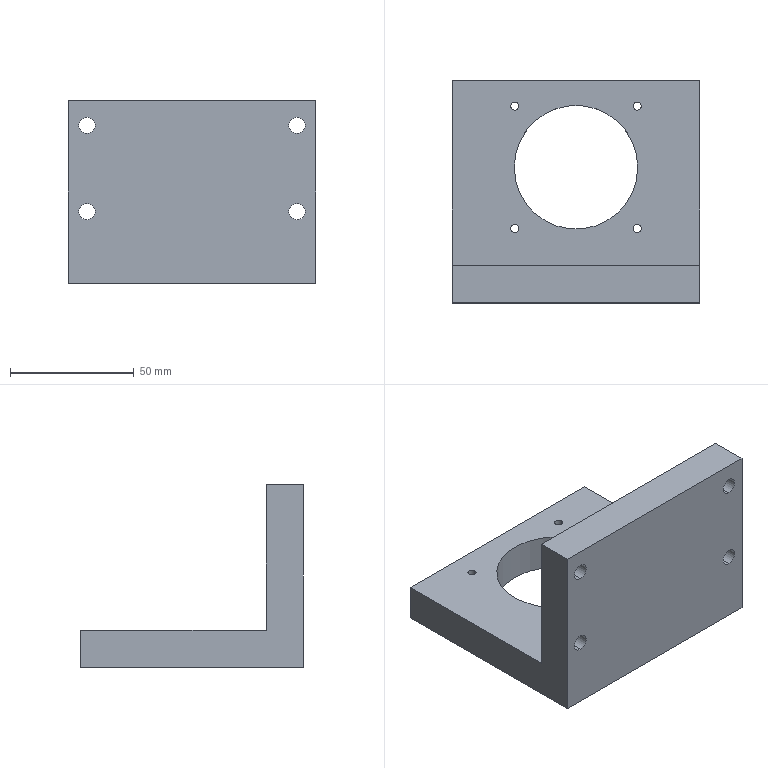Part | SolidWorks | features BaseBody 1 | 1 solid | 46 faces | box 100 x 90 x 74 mm | volume 189827 mm3 | cylinder 26 | plane 12 | cone 8 | commonest cylinder face diameters 3.3 x8 6.6 x8 11 x8 50 x2
STEP:
#1=CARTESIAN_POINT('',(26.399,34.749,0.));
#2=VERTEX_POINT('',#1);
#3=CARTESIAN_POINT('',(23.099,34.749,0.));
#4=VERTEX_POINT('',#3);
#5=CARTESIAN_POINT('',(24.749,34.749,0.));
#6=DIRECTION('',(0.,0.,-1.));
#7=DIRECTION('',(1.,0.,0.));
#8=AXIS2_PLACEMENT_3D('',#5,#6,#7);
#9=CIRCLE('',#8,1.65);
#10=EDGE_CURVE('',#2,#4,#9,.T.);
#11=ORIENTED_EDGE('',*,*,#10,.T.);
#12=CARTESIAN_POINT('',(23.099,34.749,15.));
#13=VERTEX_POINT('',#12);
#14=CARTESIAN_POINT('',(23.099,34.749,0.));
#15=DIRECTION('',(0.,0.,1.));
#16=VECTOR('',#15,1000.);
#17=LINE('',#14,#16);
#18=EDGE_CURVE('',#4,#13,#17,.T.);
#19=ORIENTED_EDGE('',*,*,#18,.T.);
#20=CARTESIAN_POINT('',(26.399,34.749,15.));
#21=VERTEX_POINT('',#20);
#22=CARTESIAN_POINT('',(24.749,34.749,15.));
#23=DIRECTION('',(0.,0.,1.));
#24=DIRECTION('',(1.,0.,0.));
#25=AXIS2_PLACEMENT_3D('',#22,#23,#24);
#26=CIRCLE('',#25,1.65);
#27=EDGE_CURVE('',#13,#21,#26,.T.);
#28=ORIENTED_EDGE('',*,*,#27,.T.);
#29=CARTESIAN_POINT('',(26.399,34.749,0.));
#30=DIRECTION('',(0.,0.,1.));
#31=VECTOR('',#30,1000.);
#32=LINE('',#29,#31);
#33=EDGE_CURVE('',#2,#21,#32,.T.);
#34=ORIENTED_EDGE('',*,*,#33,.F.);
#35=EDGE_LOOP('',(#11,#19,#28,#34));
#36=FACE_OUTER_BOUND('',#35,.T.);
#37=CARTESIAN_POINT('',(24.749,34.749,0.));
#38=DIRECTION('',(0.,0.,1.));
#39=DIRECTION('',(1.,0.,0.));
#40=AXIS2_PLACEMENT_3D('',#37,#38,#39);
#41=CYLINDRICAL_SURFACE('',#40,1.65);
#42=ADVANCED_FACE('',(#36),#41,.F.);
#43=CARTESIAN_POINT('',(25.,10.,0.));
#44=VERTEX_POINT('',#43);
#45=CARTESIAN_POINT('',(-25.,10.,0.));
#46=VERTEX_POINT('',#45);
#47=CARTESIAN_POINT('',(0.,10.,0.));
#48=DIRECTION('',(0.,0.,-1.));
#49=DIRECTION('',(1.,0.,0.));
#50=AXIS2_PLACEMENT_3D('',#47,#48,#49);
#51=CIRCLE('',#50,25.);
#52=EDGE_CURVE('',#44,#46,#51,.T.);
#53=ORIENTED_EDGE('',*,*,#52,.T.);
#54=CARTESIAN_POINT('',(-25.,10.,15.));
#55=VERTEX_POINT('',#54);
#56=CARTESIAN_POINT('',(-25.,10.,0.));
#57=DIRECTION('',(0.,0.,1.));
#58=VECTOR('',#57,1000.);
#59=LINE('',#56,#58);
#60=EDGE_CURVE('',#46,#55,#59,.T.);
#61=ORIENTED_EDGE('',*,*,#60,.T.);
#62=CARTESIAN_POINT('',(25.,10.,15.));
#63=VERTEX_POINT('',#62);
#64=CARTESIAN_POINT('',(0.,10.,15.));
#65=DIRECTION('',(0.,0.,-1.));
#66=DIRECTION('',(1.,0.,0.));
#67=AXIS2_PLACEMENT_3D('',#64,#65,#66);
#68=CIRCLE('',#67,25.);
#69=EDGE_CURVE('',#63,#55,#68,.T.);
#70=ORIENTED_EDGE('',*,*,#69,.F.);
#71=CARTESIAN_POINT('',(25.,10.,0.));
#72=DIRECTION('',(0.,0.,1.));
#73=VECTOR('',#72,1000.);
#74=LINE('',#71,#73);
#75=EDGE_CURVE('',#44,#63,#74,.T.);
#76=ORIENTED_EDGE('',*,*,#75,.F.);
#77=EDGE_LOOP('',(#53,#61,#70,#76));
#78=FACE_OUTER_BOUND('',#77,.T.);
#79=CARTESIAN_POINT('',(0.,10.,0.));
#80=DIRECTION('',(0.,0.,1.));
#81=DIRECTION('',(1.,0.,0.));
#82=AXIS2_PLACEMENT_3D('',#79,#80,#81);
#83=CYLINDRICAL_SURFACE('',#82,25.);
#84=ADVANCED_FACE('',(#78),#83,.F.);
#85=CARTESIAN_POINT('',(26.399,-14.749,0.));
#86=VERTEX_POINT('',#85);
#87=CARTESIAN_POINT('',(23.099,-14.749,0.));
#88=VERTEX_POINT('',#87);
#89=CARTESIAN_POINT('',(24.749,-14.749,0.));
#90=DIRECTION('',(0.,0.,-1.));
#91=DIRECTION('',(1.,0.,0.));
#92=AXIS2_PLACEMENT_3D('',#89,#90,#91);
#93=CIRCLE('',#92,1.65);
#94=EDGE_CURVE('',#86,#88,#93,.T.);
#95=ORIENTED_EDGE('',*,*,#94,.T.);
#96=CARTESIAN_POINT('',(23.099,-14.749,15.));
#97=VERTEX_POINT('',#96);
#98=CARTESIAN_POINT('',(23.099,-14.749,0.));
#99=DIRECTION('',(0.,0.,1.));
#100=VECTOR('',#99,1000.);
#101=LINE('',#98,#100);
#102=EDGE_CURVE('',#88,#97,#101,.T.);
#103=ORIENTED_EDGE('',*,*,#102,.T.);
#104=CARTESIAN_POINT('',(26.399,-14.749,15.));
#105=VERTEX_POINT('',#104);
#106=CARTESIAN_POINT('',(24.749,-14.749,15.));
#107=DIRECTION('',(0.,0.,-1.));
#108=DIRECTION('',(1.,0.,0.));
#109=AXIS2_PLACEMENT_3D('',#106,#107,#108);
#110=CIRCLE('',#109,1.65);
#111=EDGE_CURVE('',#105,#97,#110,.T.);
#112=ORIENTED_EDGE('',*,*,#111,.F.);
#113=CARTESIAN_POINT('',(26.399,-14.749,0.));
#114=DIRECTION('',(0.,0.,1.));
#115=VECTOR('',#114,1000.);
#116=LINE('',#113,#115);
#117=EDGE_CURVE('',#86,#105,#116,.T.);
#118=ORIENTED_EDGE('',*,*,#117,.F.);
#119=EDGE_LOOP('',(#95,#103,#112,#118));
#120=FACE_OUTER_BOUND('',#119,.T.);
#121=CARTESIAN_POINT('',(24.749,-14.749,0.));
#122=DIRECTION('',(0.,0.,1.));
#123=DIRECTION('',(1.,0.,0.));
#124=AXIS2_PLACEMENT_3D('',#121,#122,#123);
#125=CYLINDRICAL_SURFACE('',#124,1.65);
#126=ADVANCED_FACE('',(#120),#125,.F.);
#127=CARTESIAN_POINT('',(-23.099,-14.749,0.));
#128=VERTEX_POINT('',#127);
#129=CARTESIAN_POINT('',(-26.399,-14.749,0.));
#130=VERTEX_POINT('',#129);
#131=CARTESIAN_POINT('',(-24.749,-14.749,0.));
#132=DIRECTION('',(0.,0.,-1.));
#133=DIRECTION('',(1.,0.,0.));
#134=AXIS2_PLACEMENT_3D('',#131,#132,#133);
#135=CIRCLE('',#134,1.65);
#136=EDGE_CURVE('',#128,#130,#135,.T.);
#137=ORIENTED_EDGE('',*,*,#136,.T.);
#138=CARTESIAN_POINT('',(-26.399,-14.749,15.));
#139=VERTEX_POINT('',#138);
#140=CARTESIAN_POINT('',(-26.399,-14.749,0.));
#141=DIRECTION('',(0.,0.,1.));
#142=VECTOR('',#141,1000.);
#143=LINE('',#140,#142);
#144=EDGE_CURVE('',#130,#139,#143,.T.);
#145=ORIENTED_EDGE('',*,*,#144,.T.);
#146=CARTESIAN_POINT('',(-23.099,-14.749,15.));
#147=VERTEX_POINT('',#146);
#148=CARTESIAN_POINT('',(-24.749,-14.749,15.));
#149=DIRECTION('',(0.,0.,-1.));
#150=DIRECTION('',(1.,0.,0.));
#151=AXIS2_PLACEMENT_3D('',#148,#149,#150);
#152=CIRCLE('',#151,1.65);
#153=EDGE_CURVE('',#147,#139,#152,.T.);
#154=ORIENTED_EDGE('',*,*,#153,.F.);
#155=CARTESIAN_POINT('',(-23.099,-14.749,0.));
#156=DIRECTION('',(0.,0.,1.));
#157=VECTOR('',#156,1000.);
#158=LINE('',#155,#157);
#159=EDGE_CURVE('',#128,#147,#158,.T.);
#160=ORIENTED_EDGE('',*,*,#159,.F.);
#161=EDGE_LOOP('',(#137,#145,#154,#160));
#162=FACE_OUTER_BOUND('',#161,.T.);
#163=CARTESIAN_POINT('',(-24.749,-14.749,0.));
#164=DIRECTION('',(0.,0.,1.));
#165=DIRECTION('',(1.,0.,0.));
#166=AXIS2_PLACEMENT_3D('',#163,#164,#165);
#167=CYLINDRICAL_SURFACE('',#166,1.65);
#168=ADVANCED_FACE('',(#162),#167,.F.);
#169=CARTESIAN_POINT('',(-23.099,34.749,0.));
#170=VERTEX_POINT('',#169);
#171=CARTESIAN_POINT('',(-26.399,34.749,0.));
#172=VERTEX_POINT('',#171);
#173=CARTESIAN_POINT('',(-24.749,34.749,0.));
#174=DIRECTION('',(0.,0.,-1.));
#175=DIRECTION('',(1.,0.,0.));
#176=AXIS2_PLACEMENT_3D('',#173,#174,#175);
#177=CIRCLE('',#176,1.65);
#178=EDGE_CURVE('',#170,#172,#177,.T.);
#179=ORIENTED_EDGE('',*,*,#178,.T.);
#180=CARTESIAN_POINT('',(-26.399,34.749,15.));
#181=VERTEX_POINT('',#180);
#182=CARTESIAN_POINT('',(-26.399,34.749,0.));
#183=DIRECTION('',(0.,0.,1.));
#184=VECTOR('',#183,1000.);
#185=LINE('',#182,#184);
#186=EDGE_CURVE('',#172,#181,#185,.T.);
#187=ORIENTED_EDGE('',*,*,#186,.T.);
#188=CARTESIAN_POINT('',(-23.099,34.749,15.));
#189=VERTEX_POINT('',#188);
#190=CARTESIAN_POINT('',(-24.749,34.749,15.));
#191=DIRECTION('',(0.,0.,-1.));
#192=DIRECTION('',(1.,0.,0.));
#193=AXIS2_PLACEMENT_3D('',#190,#191,#192);
#194=CIRCLE('',#193,1.65);
#195=EDGE_CURVE('',#189,#181,#194,.T.);
#196=ORIENTED_EDGE('',*,*,#195,.F.);
#197=CARTESIAN_POINT('',(-23.099,34.749,0.));
#198=DIRECTION('',(0.,0.,1.));
#199=VECTOR('',#198,1000.);
#200=LINE('',#197,#199);
#201=EDGE_CURVE('',#170,#189,#200,.T.);
#202=ORIENTED_EDGE('',*,*,#201,.F.);
#203=EDGE_LOOP('',(#179,#187,#196,#202));
#204=FACE_OUTER_BOUND('',#203,.T.);
#205=CARTESIAN_POINT('',(-24.749,34.749,0.));
#206=DIRECTION('',(0.,0.,1.));
#207=DIRECTION('',(1.,0.,0.));
#208=AXIS2_PLACEMENT_3D('',#205,#206,#207);
#209=CYLINDRICAL_SURFACE('',#208,1.65);
#210=ADVANCED_FACE('',(#204),#209,.F.);
#211=CARTESIAN_POINT('',(42.5,-30.025,23.5));
#212=VERTEX_POINT('',#211);
#213=CARTESIAN_POINT('',(48.,-30.025,29.));
#214=VERTEX_POINT('',#213);
#215=CARTESIAN_POINT('',(42.5,-30.025,29.));
#216=DIRECTION('',(0.,-1.,0.));
#217=DIRECTION('',(0.,0.,1.));
#218=AXIS2_PLACEMENT_3D('',#215,#216,#217);
#219=CIRCLE('',#218,5.5);
#220=EDGE_CURVE('',#212,#214,#219,.T.);
#221=ORIENTED_EDGE('',*,*,#220,.T.);
#222=CARTESIAN_POINT('',(48.025,-30.,29.));
#223=VERTEX_POINT('',#222);
#224=CARTESIAN_POINT('',(48.,-30.025,29.));
#225=DIRECTION('',(0.7071,0.7071,0.));
#226=VECTOR('',#225,1000.);
#227=LINE('',#224,#226);
#228=EDGE_CURVE('',#214,#223,#227,.T.);
#229=ORIENTED_EDGE('',*,*,#228,.T.);
#230=CARTESIAN_POINT('',(36.975,-30.,29.));
#231=VERTEX_POINT('',#230);
#232=CARTESIAN_POINT('',(42.5,-30.,29.));
#233=DIRECTION('',(0.,1.,0.));
#234=DIRECTION('',(-1.,0.,0.));
#235=AXIS2_PLACEMENT_3D('',#232,#233,#234);
#236=CIRCLE('',#235,5.525);
#237=EDGE_CURVE('',#223,#231,#236,.T.);
#238=ORIENTED_EDGE('',*,*,#237,.T.);
#239=CARTESIAN_POINT('',(37.,-30.025,29.));
#240=VERTEX_POINT('',#239);
#241=CARTESIAN_POINT('',(37.,-30.025,29.));
#242=DIRECTION('',(-0.7071,0.7071,0.));
#243=VECTOR('',#242,1000.);
#244=LINE('',#241,#243);
#245=EDGE_CURVE('',#240,#231,#244,.T.);
#246=ORIENTED_EDGE('',*,*,#245,.F.);
#247=CARTESIAN_POINT('',(42.5,-30.025,29.));
#248=DIRECTION('',(0.,-1.,0.));
#249=DIRECTION('',(0.,0.,1.));
#250=AXIS2_PLACEMENT_3D('',#247,#248,#249);
#251=CIRCLE('',#250,5.5);
#252=EDGE_CURVE('',#240,#212,#251,.T.);
#253=ORIENTED_EDGE('',*,*,#252,.T.);
#254=EDGE_LOOP('',(#221,#229,#238,#246,#253));
#255=FACE_OUTER_BOUND('',#254,.T.);
#256=CARTESIAN_POINT('',(42.5,-30.025,29.));
#257=DIRECTION('',(0.,1.,0.));
#258=DIRECTION('',(-1.,0.,0.));
#259=AXIS2_PLACEMENT_3D('',#256,#257,#258);
#260=CONICAL_SURFACE('',#259,5.5,0.7854);
#261=ADVANCED_FACE('',(#255),#260,.F.);
#262=CARTESIAN_POINT('',(42.5,-30.025,58.5));
#263=VERTEX_POINT('',#262);
#264=CARTESIAN_POINT('',(48.,-30.025,64.));
#265=VERTEX_POINT('',#264);
#266=CARTESIAN_POINT('',(42.5,-30.025,64.));
#267=DIRECTION('',(0.,-1.,0.));
#268=DIRECTION('',(0.,0.,1.));
#269=AXIS2_PLACEMENT_3D('',#266,#267,#268);
#270=CIRCLE('',#269,5.5);
#271=EDGE_CURVE('',#263,#265,#270,.T.);
#272=ORIENTED_EDGE('',*,*,#271,.T.);
#273=CARTESIAN_POINT('',(48.025,-30.,64.));
#274=VERTEX_POINT('',#273);
#275=CARTESIAN_POINT('',(48.,-30.025,64.));
#276=DIRECTION('',(0.7071,0.7071,0.));
#277=VECTOR('',#276,1000.);
#278=LINE('',#275,#277);
#279=EDGE_CURVE('',#265,#274,#278,.T.);
#280=ORIENTED_EDGE('',*,*,#279,.T.);
#281=CARTESIAN_POINT('',(36.975,-30.,64.));
#282=VERTEX_POINT('',#281);
#283=CARTESIAN_POINT('',(42.5,-30.,64.));
#284=DIRECTION('',(0.,1.,0.));
#285=DIRECTION('',(-1.,0.,0.));
#286=AXIS2_PLACEMENT_3D('',#283,#284,#285);
#287=CIRCLE('',#286,5.525);
#288=EDGE_CURVE('',#274,#282,#287,.T.);
#289=ORIENTED_EDGE('',*,*,#288,.T.);
#290=CARTESIAN_POINT('',(37.,-30.025,64.));
#291=VERTEX_POINT('',#290);
#292=CARTESIAN_POINT('',(37.,-30.025,64.));
#293=DIRECTION('',(-0.7071,0.7071,0.));
#294=VECTOR('',#293,1000.);
#295=LINE('',#292,#294);
#296=EDGE_CURVE('',#291,#282,#295,.T.);
#297=ORIENTED_EDGE('',*,*,#296,.F.);
#298=CARTESIAN_POINT('',(42.5,-30.025,64.));
#299=DIRECTION('',(0.,-1.,0.));
#300=DIRECTION('',(0.,0.,1.));
#301=AXIS2_PLACEMENT_3D('',#298,#299,#300);
#302=CIRCLE('',#301,5.5);
#303=EDGE_CURVE('',#291,#263,#302,.T.);
#304=ORIENTED_EDGE('',*,*,#303,.T.);
#305=EDGE_LOOP('',(#272,#280,#289,#297,#304));
#306=FACE_OUTER_BOUND('',#305,.T.);
#307=CARTESIAN_POINT('',(42.5,-30.025,64.));
#308=DIRECTION('',(0.,1.,0.));
#309=DIRECTION('',(-1.,0.,0.));
#310=AXIS2_PLACEMENT_3D('',#307,#308,#309);
#311=CONICAL_SURFACE('',#310,5.5,0.7854);
#312=ADVANCED_FACE('',(#306),#311,.F.);
#313=CARTESIAN_POINT('',(-42.5,-30.025,58.5));
#314=VERTEX_POINT('',#313);
#315=CARTESIAN_POINT('',(-37.,-30.025,64.));
#316=VERTEX_POINT('',#315);
#317=CARTESIAN_POINT('',(-42.5,-30.025,64.));
#318=DIRECTION('',(0.,-1.,0.));
#319=DIRECTION('',(0.,0.,1.));
#320=AXIS2_PLACEMENT_3D('',#317,#318,#319);
#321=CIRCLE('',#320,5.5);
#322=EDGE_CURVE('',#314,#316,#321,.T.);
#323=ORIENTED_EDGE('',*,*,#322,.T.);
#324=CARTESIAN_POINT('',(-36.975,-30.,64.));
#325=VERTEX_POINT('',#324);
#326=CARTESIAN_POINT('',(-37.,-30.025,64.));
#327=DIRECTION('',(0.7071,0.7071,0.));
#328=VECTOR('',#327,1000.);
#329=LINE('',#326,#328);
#330=EDGE_CURVE('',#316,#325,#329,.T.);
#331=ORIENTED_EDGE('',*,*,#330,.T.);
#332=CARTESIAN_POINT('',(-48.025,-30.,64.));
#333=VERTEX_POINT('',#332);
#334=CARTESIAN_POINT('',(-42.5,-30.,64.));
#335=DIRECTION('',(0.,1.,0.));
#336=DIRECTION('',(-1.,0.,0.));
#337=AXIS2_PLACEMENT_3D('',#334,#335,#336);
#338=CIRCLE('',#337,5.525);
#339=EDGE_CURVE('',#325,#333,#338,.T.);
#340=ORIENTED_EDGE('',*,*,#339,.T.);
#341=CARTESIAN_POINT('',(-48.,-30.025,64.));
#342=VERTEX_POINT('',#341);
#343=CARTESIAN_POINT('',(-48.,-30.025,64.));
#344=DIRECTION('',(-0.7071,0.7071,0.));
#345=VECTOR('',#344,1000.);
#346=LINE('',#343,#345);
#347=EDGE_CURVE('',#342,#333,#346,.T.);
#348=ORIENTED_EDGE('',*,*,#347,.F.);
#349=CARTESIAN_POINT('',(-42.5,-30.025,64.));
#350=DIRECTION('',(0.,-1.,0.));
#351=DIRECTION('',(0.,0.,1.));
#352=AXIS2_PLACEMENT_3D('',#349,#350,#351);
#353=CIRCLE('',#352,5.5);
#354=EDGE_CURVE('',#342,#314,#353,.T.);
#355=ORIENTED_EDGE('',*,*,#354,.T.);
#356=EDGE_LOOP('',(#323,#331,#340,#348,#355));
#357=FACE_OUTER_BOUND('',#356,.T.);
#358=CARTESIAN_POINT('',(-42.5,-30.025,64.));
#359=DIRECTION('',(0.,1.,0.));
#360=DIRECTION('',(-1.,0.,0.));
#361=AXIS2_PLACEMENT_3D('',#358,#359,#360);
#362=CONICAL_SURFACE('',#361,5.5,0.7854);
#363=ADVANCED_FACE('',(#357),#362,.F.);
#364=CARTESIAN_POINT('',(-42.5,-30.025,23.5));
#365=VERTEX_POINT('',#364);
#366=CARTESIAN_POINT('',(-37.,-30.025,29.));
#367=VERTEX_POINT('',#366);
#368=CARTESIAN_POINT('',(-42.5,-30.025,29.));
#369=DIRECTION('',(0.,-1.,0.));
#370=DIRECTION('',(0.,0.,1.));
#371=AXIS2_PLACEMENT_3D('',#368,#369,#370);
#372=CIRCLE('',#371,5.5);
#373=EDGE_CURVE('',#365,#367,#372,.T.);
#374=ORIENTED_EDGE('',*,*,#373,.T.);
#375=CARTESIAN_POINT('',(-36.975,-30.,29.));
#376=VERTEX_POINT('',#375);
#377=CARTESIAN_POINT('',(-37.,-30.025,29.));
#378=DIRECTION('',(0.7071,0.7071,0.));
#379=VECTOR('',#378,1000.);
#380=LINE('',#377,#379);
#381=EDGE_CURVE('',#367,#376,#380,.T.);
#382=ORIENTED_EDGE('',*,*,#381,.T.);
#383=CARTESIAN_POINT('',(-48.025,-30.,29.));
#384=VERTEX_POINT('',#383);
#385=CARTESIAN_POINT('',(-42.5,-30.,29.));
#386=DIRECTION('',(0.,1.,0.));
#387=DIRECTION('',(-1.,0.,0.));
#388=AXIS2_PLACEMENT_3D('',#385,#386,#387);
#389=CIRCLE('',#388,5.525);
#390=EDGE_CURVE('',#376,#384,#389,.T.);
#391=ORIENTED_EDGE('',*,*,#390,.T.);
#392=CARTESIAN_POINT('',(-48.,-30.025,29.));
#393=VERTEX_POINT('',#392);
#394=CARTESIAN_POINT('',(-48.,-30.025,29.));
#395=DIRECTION('',(-0.7071,0.7071,0.));
#396=VECTOR('',#395,1000.);
#397=LINE('',#394,#396);
#398=EDGE_CURVE('',#393,#384,#397,.T.);
#399=ORIENTED_EDGE('',*,*,#398,.F.);
#400=CARTESIAN_POINT('',(-42.5,-30.025,29.));
#401=DIRECTION('',(0.,-1.,0.));
#402=DIRECTION('',(0.,0.,1.));
#403=AXIS2_PLACEMENT_3D('',#400,#401,#402);
#404=CIRCLE('',#403,5.5);
#405=EDGE_CURVE('',#393,#365,#404,.T.);
#406=ORIENTED_EDGE('',*,*,#405,.T.);
#407=EDGE_LOOP('',(#374,#382,#391,#399,#406));
#408=FACE_OUTER_BOUND('',#407,.T.);
#409=CARTESIAN_POINT('',(-42.5,-30.025,29.));
#410=DIRECTION('',(0.,1.,0.));
#411=DIRECTION('',(-1.,0.,0.));
#412=AXIS2_PLACEMENT_3D('',#409,#410,#411);
#413=CONICAL_SURFACE('',#412,5.5,0.7854);
#414=ADVANCED_FACE('',(#408),#413,.F.);
#415=CARTESIAN_POINT('',(42.5,-45.,32.3));
#416=VERTEX_POINT('',#415);
#417=CARTESIAN_POINT('',(42.5,-45.,25.7));
#418=VERTEX_POINT('',#417);
#419=CARTESIAN_POINT('',(42.5,-45.,29.));
#420=DIRECTION('',(0.,-1.,0.));
#421=DIRECTION('',(0.,0.,1.));
#422=AXIS2_PLACEMENT_3D('',#419,#420,#421);
#423=CIRCLE('',#422,3.3);
#424=EDGE_CURVE('',#416,#418,#423,.T.);
#425=ORIENTED_EDGE('',*,*,#424,.T.);
#426=CARTESIAN_POINT('',(42.5,-36.8,25.7));
#427=VERTEX_POINT('',#426);
#428=CARTESIAN_POINT('',(42.5,-45.,25.7));
#429=DIRECTION('',(0.,1.,0.));
#430=VECTOR('',#429,1000.);
#431=LINE('',#428,#430);
#432=EDGE_CURVE('',#418,#427,#431,.T.);
#433=ORIENTED_EDGE('',*,*,#432,.T.);
#434=CARTESIAN_POINT('',(42.5,-36.8,32.3));
#435=VERTEX_POINT('',#434);
#436=CARTESIAN_POINT('',(42.5,-36.8,29.));
#437=DIRECTION('',(0.,1.,0.));
#438=DIRECTION('',(0.,0.,1.));
#439=AXIS2_PLACEMENT_3D('',#436,#437,#438);
#440=CIRCLE('',#439,3.3);
#441=EDGE_CURVE('',#427,#435,#440,.T.);
#442=ORIENTED_EDGE('',*,*,#441,.T.);
#443=CARTESIAN_POINT('',(42.5,-45.,32.3));
#444=DIRECTION('',(0.,1.,0.));
#445=VECTOR('',#444,1000.);
#446=LINE('',#443,#445);
#447=EDGE_CURVE('',#416,#435,#446,.T.);
#448=ORIENTED_EDGE('',*,*,#447,.F.);
#449=EDGE_LOOP('',(#425,#433,#442,#448));
#450=FACE_OUTER_BOUND('',#449,.T.);
#451=CARTESIAN_POINT('',(42.5,-45.,29.));
#452=DIRECTION('',(0.,1.,0.));
#453=DIRECTION('',(0.,0.,1.));
#454=AXIS2_PLACEMENT_3D('',#451,#452,#453);
#455=CYLINDRICAL_SURFACE('',#454,3.3);
#456=ADVANCED_FACE('',(#450),#455,.F.);
#457=CARTESIAN_POINT('',(42.5,-45.,67.3));
#458=VERTEX_POINT('',#457);
#459=CARTESIAN_POINT('',(42.5,-45.,60.7));
#460=VERTEX_POINT('',#459);
#461=CARTESIAN_POINT('',(42.5,-45.,64.));
#462=DIRECTION('',(0.,-1.,0.));
#463=DIRECTION('',(0.,0.,1.));
#464=AXIS2_PLACEMENT_3D('',#461,#462,#463);
#465=CIRCLE('',#464,3.3);
#466=EDGE_CURVE('',#458,#460,#465,.T.);
#467=ORIENTED_EDGE('',*,*,#466,.T.);
#468=CARTESIAN_POINT('',(42.5,-36.8,60.7));
#469=VERTEX_POINT('',#468);
#470=CARTESIAN_POINT('',(42.5,-45.,60.7));
#471=DIRECTION('',(0.,1.,0.));
#472=VECTOR('',#471,1000.);
#473=LINE('',#470,#472);
#474=EDGE_CURVE('',#460,#469,#473,.T.);
#475=ORIENTED_EDGE('',*,*,#474,.T.);
#476=CARTESIAN_POINT('',(42.5,-36.8,67.3));
#477=VERTEX_POINT('',#476);
#478=CARTESIAN_POINT('',(42.5,-36.8,64.));
#479=DIRECTION('',(0.,1.,0.));
#480=DIRECTION('',(0.,0.,1.));
#481=AXIS2_PLACEMENT_3D('',#478,#479,#480);
#482=CIRCLE('',#481,3.3);
#483=EDGE_CURVE('',#469,#477,#482,.T.);
#484=ORIENTED_EDGE('',*,*,#483,.T.);
#485=CARTESIAN_POINT('',(42.5,-45.,67.3));
#486=DIRECTION('',(0.,1.,0.));
#487=VECTOR('',#486,1000.);
#488=LINE('',#485,#487);
#489=EDGE_CURVE('',#458,#477,#488,.T.);
#490=ORIENTED_EDGE('',*,*,#489,.F.);
#491=EDGE_LOOP('',(#467,#475,#484,#490));
#492=FACE_OUTER_BOUND('',#491,.T.);
#493=CARTESIAN_POINT('',(42.5,-45.,64.));
#494=DIRECTION('',(0.,1.,0.));
#495=DIRECTION('',(0.,0.,1.));
#496=AXIS2_PLACEMENT_3D('',#493,#494,#495);
#497=CYLINDRICAL_SURFACE('',#496,3.3);
#498=ADVANCED_FACE('',(#492),#497,.F.);
#499=CARTESIAN_POINT('',(-42.5,-45.,67.3));
#500=VERTEX_POINT('',#499);
#501=CARTESIAN_POINT('',(-42.5,-45.,60.7));
#502=VERTEX_POINT('',#501);
#503=CARTESIAN_POINT('',(-42.5,-45.,64.));
#504=DIRECTION('',(0.,-1.,0.));
#505=DIRECTION('',(0.,0.,1.));
#506=AXIS2_PLACEMENT_3D('',#503,#504,#505);
#507=CIRCLE('',#506,3.3);
#508=EDGE_CURVE('',#500,#502,#507,.T.);
#509=ORIENTED_EDGE('',*,*,#508,.T.);
#510=CARTESIAN_POINT('',(-42.5,-36.8,60.7));
#511=VERTEX_POINT('',#510);
#512=CARTESIAN_POINT('',(-42.5,-45.,60.7));
#513=DIRECTION('',(0.,1.,0.));
#514=VECTOR('',#513,1000.);
#515=LINE('',#512,#514);
#516=EDGE_CURVE('',#502,#511,#515,.T.);
#517=ORIENTED_EDGE('',*,*,#516,.T.);
#518=CARTESIAN_POINT('',(-42.5,-36.8,67.3));
#519=VERTEX_POINT('',#518);
#520=CARTESIAN_POINT('',(-42.5,-36.8,64.));
#521=DIRECTION('',(0.,1.,0.));
#522=DIRECTION('',(0.,0.,1.));
#523=AXIS2_PLACEMENT_3D('',#520,#521,#522);
#524=CIRCLE('',#523,3.3);
#525=EDGE_CURVE('',#511,#519,#524,.T.);
#526=ORIENTED_EDGE('',*,*,#525,.T.);
#527=CARTESIAN_POINT('',(-42.5,-45.,67.3));
#528=DIRECTION('',(0.,1.,0.));
#529=VECTOR('',#528,1000.);
#530=LINE('',#527,#529);
#531=EDGE_CURVE('',#500,#519,#530,.T.);
#532=ORIENTED_EDGE('',*,*,#531,.F.);
#533=EDGE_LOOP('',(#509,#517,#526,#532));
#534=FACE_OUTER_BOUND('',#533,.T.);
#535=CARTESIAN_POINT('',(-42.5,-45.,64.));
#536=DIRECTION('',(0.,1.,0.));
#537=DIRECTION('',(0.,0.,1.));
#538=AXIS2_PLACEMENT_3D('',#535,#536,#537);
#539=CYLINDRICAL_SURFACE('',#538,3.3);
#540=ADVANCED_FACE('',(#534),#539,.F.);
#541=CARTESIAN_POINT('',(-42.5,-45.,32.3));
#542=VERTEX_POINT('',#541);
#543=CARTESIAN_POINT('',(-42.5,-45.,25.7));
#544=VERTEX_POINT('',#543);
#545=CARTESIAN_POINT('',(-42.5,-45.,29.));
#546=DIRECTION('',(0.,-1.,0.));
#547=DIRECTION('',(0.,0.,1.));
#548=AXIS2_PLACEMENT_3D('',#545,#546,#547);
#549=CIRCLE('',#548,3.3);
#550=EDGE_CURVE('',#542,#544,#549,.T.);
#551=ORIENTED_EDGE('',*,*,#550,.T.);
#552=CARTESIAN_POINT('',(-42.5,-36.8,25.7));
#553=VERTEX_POINT('',#552);
#554=CARTESIAN_POINT('',(-42.5,-45.,25.7));
#555=DIRECTION('',(0.,1.,0.));
#556=VECTOR('',#555,1000.);
#557=LINE('',#554,#556);
#558=EDGE_CURVE('',#544,#553,#557,.T.);
#559=ORIENTED_EDGE('',*,*,#558,.T.);
#560=CARTESIAN_POINT('',(-42.5,-36.8,32.3));
#561=VERTEX_POINT('',#560);
#562=CARTESIAN_POINT('',(-42.5,-36.8,29.));
#563=DIRECTION('',(0.,1.,0.));
#564=DIRECTION('',(0.,0.,1.));
#565=AXIS2_PLACEMENT_3D('',#562,#563,#564);
#566=CIRCLE('',#565,3.3);
#567=EDGE_CURVE('',#553,#561,#566,.T.);
#568=ORIENTED_EDGE('',*,*,#567,.T.);
#569=CARTESIAN_POINT('',(-42.5,-45.,32.3));
#570=DIRECTION('',(0.,1.,0.));
#571=VECTOR('',#570,1000.);
#572=LINE('',#569,#571);
#573=EDGE_CURVE('',#542,#561,#572,.T.);
#574=ORIENTED_EDGE('',*,*,#573,.F.);
#575=EDGE_LOOP('',(#551,#559,#568,#574));
#576=FACE_OUTER_BOUND('',#575,.T.);
#577=CARTESIAN_POINT('',(-42.5,-45.,29.));
#578=DIRECTION('',(0.,1.,0.));
#579=DIRECTION('',(0.,0.,1.));
#580=AXIS2_PLACEMENT_3D('',#577,#578,#579);
#581=CYLINDRICAL_SURFACE('',#580,3.3);
#582=ADVANCED_FACE('',(#576),#581,.F.);
#583=CARTESIAN_POINT('',(42.5,-36.8,34.5));
#584=VERTEX_POINT('',#583);
#585=CARTESIAN_POINT('',(42.5,-36.8,23.5));
#586=VERTEX_POINT('',#585);
#587=CARTESIAN_POINT('',(42.5,-36.8,29.));
#588=DIRECTION('',(0.,-1.,0.));
#589=DIRECTION('',(0.,0.,1.));
#590=AXIS2_PLACEMENT_3D('',#587,#588,#589);
#591=CIRCLE('',#590,5.5);
#592=EDGE_CURVE('',#584,#586,#591,.T.);
#593=ORIENTED_EDGE('',*,*,#592,.T.);
#594=CARTESIAN_POINT('',(42.5,-36.8,23.5));
#595=DIRECTION('',(0.,1.,0.));
#596=VECTOR('',#595,1000.);
#597=LINE('',#594,#596);
#598=EDGE_CURVE('',#586,#212,#597,.T.);
#599=ORIENTED_EDGE('',*,*,#598,.T.);
#600=ORIENTED_EDGE('',*,*,#252,.F.);
#601=CARTESIAN_POINT('',(42.5,-30.025,34.5));
#602=VERTEX_POINT('',#601);
#603=CARTESIAN_POINT('',(42.5,-30.025,29.));
#604=DIRECTION('',(0.,-1.,0.));
#605=DIRECTION('',(0.,0.,1.));
#606=AXIS2_PLACEMENT_3D('',#603,#604,#605);
#607=CIRCLE('',#606,5.5);
#608=EDGE_CURVE('',#602,#240,#607,.T.);
#609=ORIENTED_EDGE('',*,*,#608,.F.);
#610=CARTESIAN_POINT('',(42.5,-36.8,34.5));
#611=DIRECTION('',(0.,1.,0.));
#612=VECTOR('',#611,1000.);
#613=LINE('',#610,#612);
#614=EDGE_CURVE('',#584,#602,#613,.T.);
#615=ORIENTED_EDGE('',*,*,#614,.F.);
#616=EDGE_LOOP('',(#593,#599,#600,#609,#615));
#617=FACE_OUTER_BOUND('',#616,.T.);
#618=CARTESIAN_POINT('',(42.5,-36.8,29.));
#619=DIRECTION('',(0.,1.,0.));
#620=DIRECTION('',(0.,0.,1.));
#621=AXIS2_PLACEMENT_3D('',#618,#619,#620);
#622=CYLINDRICAL_SURFACE('',#621,5.5);
#623=ADVANCED_FACE('',(#617),#622,.F.);
#624=CARTESIAN_POINT('',(42.5,-36.8,69.5));
#625=VERTEX_POINT('',#624);
#626=CARTESIAN_POINT('',(42.5,-36.8,58.5));
#627=VERTEX_POINT('',#626);
#628=CARTESIAN_POINT('',(42.5,-36.8,64.));
#629=DIRECTION('',(0.,-1.,0.));
#630=DIRECTION('',(0.,0.,1.));
#631=AXIS2_PLACEMENT_3D('',#628,#629,#630);
#632=CIRCLE('',#631,5.5);
#633=EDGE_CURVE('',#625,#627,#632,.T.);
#634=ORIENTED_EDGE('',*,*,#633,.T.);
#635=CARTESIAN_POINT('',(42.5,-36.8,58.5));
#636=DIRECTION('',(0.,1.,0.));
#637=VECTOR('',#636,1000.);
#638=LINE('',#635,#637);
#639=EDGE_CURVE('',#627,#263,#638,.T.);
#640=ORIENTED_EDGE('',*,*,#639,.T.);
#641=ORIENTED_EDGE('',*,*,#303,.F.);
#642=CARTESIAN_POINT('',(42.5,-30.025,69.5));
#643=VERTEX_POINT('',#642);
#644=CARTESIAN_POINT('',(42.5,-30.025,64.));
#645=DIRECTION('',(0.,-1.,0.));
#646=DIRECTION('',(0.,0.,1.));
#647=AXIS2_PLACEMENT_3D('',#644,#645,#646);
#648=CIRCLE('',#647,5.5);
#649=EDGE_CURVE('',#643,#291,#648,.T.);
#650=ORIENTED_EDGE('',*,*,#649,.F.);
#651=CARTESIAN_POINT('',(42.5,-36.8,69.5));
#652=DIRECTION('',(0.,1.,0.));
#653=VECTOR('',#652,1000.);
#654=LINE('',#651,#653);
#655=EDGE_CURVE('',#625,#643,#654,.T.);
#656=ORIENTED_EDGE('',*,*,#655,.F.);
#657=EDGE_LOOP('',(#634,#640,#641,#650,#656));
#658=FACE_OUTER_BOUND('',#657,.T.);
#659=CARTESIAN_POINT('',(42.5,-36.8,64.));
#660=DIRECTION('',(0.,1.,0.));
#661=DIRECTION('',(0.,0.,1.));
#662=AXIS2_PLACEMENT_3D('',#659,#660,#661);
#663=CYLINDRICAL_SURFACE('',#662,5.5);
#664=ADVANCED_FACE('',(#658),#663,.F.);
#665=CARTESIAN_POINT('',(-42.5,-36.8,69.5));
#666=VERTEX_POINT('',#665);
#667=CARTESIAN_POINT('',(-42.5,-36.8,58.5));
#668=VERTEX_POINT('',#667);
#669=CARTESIAN_POINT('',(-42.5,-36.8,64.));
#670=DIRECTION('',(0.,-1.,0.));
#671=DIRECTION('',(0.,0.,1.));
#672=AXIS2_PLACEMENT_3D('',#669,#670,#671);
#673=CIRCLE('',#672,5.5);
#674=EDGE_CURVE('',#666,#668,#673,.T.);
#675=ORIENTED_EDGE('',*,*,#674,.T.);
#676=CARTESIAN_POINT('',(-42.5,-36.8,58.5));
#677=DIRECTION('',(0.,1.,0.));
#678=VECTOR('',#677,1000.);
#679=LINE('',#676,#678);
#680=EDGE_CURVE('',#668,#314,#679,.T.);
#681=ORIENTED_EDGE('',*,*,#680,.T.);
#682=ORIENTED_EDGE('',*,*,#354,.F.);
#683=CARTESIAN_POINT('',(-42.5,-30.025,69.5));
#684=VERTEX_POINT('',#683);
#685=CARTESIAN_POINT('',(-42.5,-30.025,64.));
#686=DIRECTION('',(0.,-1.,0.));
#687=DIRECTION('',(0.,0.,1.));
#688=AXIS2_PLACEMENT_3D('',#685,#686,#687);
#689=CIRCLE('',#688,5.5);
#690=EDGE_CURVE('',#684,#342,#689,.T.);
#691=ORIENTED_EDGE('',*,*,#690,.F.);
#692=CARTESIAN_POINT('',(-42.5,-36.8,69.5));
#693=DIRECTION('',(0.,1.,0.));
#694=VECTOR('',#693,1000.);
#695=LINE('',#692,#694);
#696=EDGE_CURVE('',#666,#684,#695,.T.);
#697=ORIENTED_EDGE('',*,*,#696,.F.);
#698=EDGE_LOOP('',(#675,#681,#682,#691,#697));
#699=FACE_OUTER_BOUND('',#698,.T.);
#700=CARTESIAN_POINT('',(-42.5,-36.8,64.));
#701=DIRECTION('',(0.,1.,0.));
#702=DIRECTION('',(0.,0.,1.));
#703=AXIS2_PLACEMENT_3D('',#700,#701,#702);
#704=CYLINDRICAL_SURFACE('',#703,5.5);
#705=ADVANCED_FACE('',(#699),#704,.F.);
#706=CARTESIAN_POINT('',(-42.5,-36.8,34.5));
#707=VERTEX_POINT('',#706);
#708=CARTESIAN_POINT('',(-42.5,-36.8,23.5));
#709=VERTEX_POINT('',#708);
#710=CARTESIAN_POINT('',(-42.5,-36.8,29.));
#711=DIRECTION('',(0.,-1.,0.));
#712=DIRECTION('',(0.,0.,1.));
#713=AXIS2_PLACEMENT_3D('',#710,#711,#712);
#714=CIRCLE('',#713,5.5);
#715=EDGE_CURVE('',#707,#709,#714,.T.);
#716=ORIENTED_EDGE('',*,*,#715,.T.);
#717=CARTESIAN_POINT('',(-42.5,-36.8,23.5));
#718=DIRECTION('',(0.,1.,0.));
#719=VECTOR('',#718,1000.);
#720=LINE('',#717,#719);
#721=EDGE_CURVE('',#709,#365,#720,.T.);
#722=ORIENTED_EDGE('',*,*,#721,.T.);
#723=ORIENTED_EDGE('',*,*,#405,.F.);
#724=CARTESIAN_POINT('',(-42.5,-30.025,34.5));
#725=VERTEX_POINT('',#724);
#726=CARTESIAN_POINT('',(-42.5,-30.025,29.));
#727=DIRECTION('',(0.,-1.,0.));
#728=DIRECTION('',(0.,0.,1.));
#729=AXIS2_PLACEMENT_3D('',#726,#727,#728);
#730=CIRCLE('',#729,5.5);
#731=EDGE_CURVE('',#725,#393,#730,.T.);
#732=ORIENTED_EDGE('',*,*,#731,.F.);
#733=CARTESIAN_POINT('',(-42.5,-36.8,34.5));
#734=DIRECTION('',(0.,1.,0.));
#735=VECTOR('',#734,1000.);
#736=LINE('',#733,#735);
#737=EDGE_CURVE('',#707,#725,#736,.T.);
#738=ORIENTED_EDGE('',*,*,#737,.F.);
#739=EDGE_LOOP('',(#716,#722,#723,#732,#738));
#740=FACE_OUTER_BOUND('',#739,.T.);
#741=CARTESIAN_POINT('',(-42.5,-36.8,29.));
#742=DIRECTION('',(0.,1.,0.));
#743=DIRECTION('',(0.,0.,1.));
#744=AXIS2_PLACEMENT_3D('',#741,#742,#743);
#745=CYLINDRICAL_SURFACE('',#744,5.5);
#746=ADVANCED_FACE('',(#740),#745,.F.);
#747=ORIENTED_EDGE('',*,*,#18,.F.);
#748=CARTESIAN_POINT('',(24.749,34.749,0.));
#749=DIRECTION('',(0.,0.,-1.));
#750=DIRECTION('',(1.,0.,0.));
#751=AXIS2_PLACEMENT_3D('',#748,#749,#750);
#752=CIRCLE('',#751,1.65);
#753=EDGE_CURVE('',#4,#2,#752,.T.);
#754=ORIENTED_EDGE('',*,*,#753,.T.);
#755=ORIENTED_EDGE('',*,*,#33,.T.);
#756=CARTESIAN_POINT('',(24.749,34.749,15.));
#757=DIRECTION('',(0.,0.,1.));
#758=DIRECTION('',(1.,0.,0.));
#759=AXIS2_PLACEMENT_3D('',#756,#757,#758);
#760=CIRCLE('',#759,1.65);
#761=EDGE_CURVE('',#21,#13,#760,.T.);
#762=ORIENTED_EDGE('',*,*,#761,.T.);
#763=EDGE_LOOP('',(#747,#754,#755,#762));
#764=FACE_OUTER_BOUND('',#763,.T.);
#765=CARTESIAN_POINT('',(24.749,34.749,0.));
#766=DIRECTION('',(0.,0.,1.));
#767=DIRECTION('',(1.,0.,0.));
#768=AXIS2_PLACEMENT_3D('',#765,#766,#767);
#769=CYLINDRICAL_SURFACE('',#768,1.65);
#770=ADVANCED_FACE('',(#764),#769,.F.);
#771=ORIENTED_EDGE('',*,*,#69,.T.);
#772=CARTESIAN_POINT('',(0.,10.,15.));
#773=DIRECTION('',(0.,0.,-1.));
#774=DIRECTION('',(1.,0.,0.));
#775=AXIS2_PLACEMENT_3D('',#772,#773,#774);
#776=CIRCLE('',#775,25.);
#777=EDGE_CURVE('',#55,#63,#776,.T.);
#778=ORIENTED_EDGE('',*,*,#777,.T.);
#779=EDGE_LOOP('',(#771,#778));
#780=FACE_BOUND('',#779,.T.);
#781=ORIENTED_EDGE('',*,*,#111,.T.);
#782=CARTESIAN_POINT('',(24.749,-14.749,15.));
#783=DIRECTION('',(0.,0.,-1.));
#784=DIRECTION('',(1.,0.,0.));
#785=AXIS2_PLACEMENT_3D('',#782,#783,#784);
#786=CIRCLE('',#785,1.65);
#787=EDGE_CURVE('',#97,#105,#786,.T.);
#788=ORIENTED_EDGE('',*,*,#787,.T.);
#789=EDGE_LOOP('',(#781,#788));
#790=FACE_BOUND('',#789,.T.);
#791=ORIENTED_EDGE('',*,*,#153,.T.);
#792=CARTESIAN_POINT('',(-24.749,-14.749,15.));
#793=DIRECTION('',(0.,0.,-1.));
#794=DIRECTION('',(1.,0.,0.));
#795=AXIS2_PLACEMENT_3D('',#792,#793,#794);
#796=CIRCLE('',#795,1.65);
#797=EDGE_CURVE('',#139,#147,#796,.T.);
#798=ORIENTED_EDGE('',*,*,#797,.T.);
#799=EDGE_LOOP('',(#791,#798));
#800=FACE_BOUND('',#799,.T.);
#801=ORIENTED_EDGE('',*,*,#195,.T.);
#802=CARTESIAN_POINT('',(-24.749,34.749,15.));
#803=DIRECTION('',(0.,0.,-1.));
#804=DIRECTION('',(1.,0.,0.));
#805=AXIS2_PLACEMENT_3D('',#802,#803,#804);
#806=CIRCLE('',#805,1.65);
#807=EDGE_CURVE('',#181,#189,#806,.T.);
#808=ORIENTED_EDGE('',*,*,#807,.T.);
#809=EDGE_LOOP('',(#801,#808));
#810=FACE_BOUND('',#809,.T.);
#811=ORIENTED_EDGE('',*,*,#761,.F.);
#812=ORIENTED_EDGE('',*,*,#27,.F.);
#813=EDGE_LOOP('',(#811,#812));
#814=FACE_BOUND('',#813,.T.);
#815=CARTESIAN_POINT('',(50.,45.,15.));
#816=VERTEX_POINT('',#815);
#817=CARTESIAN_POINT('',(-50.,45.,15.));
#818=VERTEX_POINT('',#817);
#819=CARTESIAN_POINT('',(0.,45.,15.));
#820=DIRECTION('',(-1.,0.,0.));
#821=VECTOR('',#820,1000.);
#822=LINE('',#819,#821);
#823=EDGE_CURVE('',#816,#818,#822,.T.);
#824=ORIENTED_EDGE('',*,*,#823,.T.);
#825=CARTESIAN_POINT('',(-50.,-30.,15.));
#826=VERTEX_POINT('',#825);
#827=CARTESIAN_POINT('',(-50.,7.5,15.));
#828=DIRECTION('',(0.,-1.,0.));
#829=VECTOR('',#828,1000.);
#830=LINE('',#827,#829);
#831=EDGE_CURVE('',#818,#826,#830,.T.);
#832=ORIENTED_EDGE('',*,*,#831,.T.);
#833=CARTESIAN_POINT('',(50.,-30.,15.));
#834=VERTEX_POINT('',#833);
#835=CARTESIAN_POINT('',(0.,-30.,15.));
#836=DIRECTION('',(1.,0.,0.));
#837=VECTOR('',#836,1000.);
#838=LINE('',#835,#837);
#839=EDGE_CURVE('',#826,#834,#838,.T.);
#840=ORIENTED_EDGE('',*,*,#839,.T.);
#841=CARTESIAN_POINT('',(50.,7.5,15.));
#842=DIRECTION('',(0.,1.,0.));
#843=VECTOR('',#842,1000.);
#844=LINE('',#841,#843);
#845=EDGE_CURVE('',#834,#816,#844,.T.);
#846=ORIENTED_EDGE('',*,*,#845,.T.);
#847=EDGE_LOOP('',(#824,#832,#840,#846));
#848=FACE_OUTER_BOUND('',#847,.T.);
#849=CARTESIAN_POINT('',(-50.,-30.,15.));
#850=DIRECTION('',(0.,0.,1.));
#851=DIRECTION('',(1.,0.,0.));
#852=AXIS2_PLACEMENT_3D('',#849,#850,#851);
#853=PLANE('',#852);
#854=ADVANCED_FACE('',(#780,#790,#800,#810,#814,#848),#853,.T.);
#855=ORIENTED_EDGE('',*,*,#52,.F.);
#856=CARTESIAN_POINT('',(0.,10.,0.));
#857=DIRECTION('',(0.,0.,-1.));
#858=DIRECTION('',(1.,0.,0.));
#859=AXIS2_PLACEMENT_3D('',#856,#857,#858);
#860=CIRCLE('',#859,25.);
#861=EDGE_CURVE('',#46,#44,#860,.T.);
#862=ORIENTED_EDGE('',*,*,#861,.F.);
#863=EDGE_LOOP('',(#855,#862));
#864=FACE_BOUND('',#863,.T.);
#865=ORIENTED_EDGE('',*,*,#94,.F.);
#866=CARTESIAN_POINT('',(24.749,-14.749,0.));
#867=DIRECTION('',(0.,0.,-1.));
#868=DIRECTION('',(1.,0.,0.));
#869=AXIS2_PLACEMENT_3D('',#866,#867,#868);
#870=CIRCLE('',#869,1.65);
#871=EDGE_CURVE('',#88,#86,#870,.T.);
#872=ORIENTED_EDGE('',*,*,#871,.F.);
#873=EDGE_LOOP('',(#865,#872));
#874=FACE_BOUND('',#873,.T.);
#875=ORIENTED_EDGE('',*,*,#136,.F.);
#876=CARTESIAN_POINT('',(-24.749,-14.749,0.));
#877=DIRECTION('',(0.,0.,-1.));
#878=DIRECTION('',(1.,0.,0.));
#879=AXIS2_PLACEMENT_3D('',#876,#877,#878);
#880=CIRCLE('',#879,1.65);
#881=EDGE_CURVE('',#130,#128,#880,.T.);
#882=ORIENTED_EDGE('',*,*,#881,.F.);
#883=EDGE_LOOP('',(#875,#882));
#884=FACE_BOUND('',#883,.T.);
#885=ORIENTED_EDGE('',*,*,#178,.F.);
#886=CARTESIAN_POINT('',(-24.749,34.749,0.));
#887=DIRECTION('',(0.,0.,-1.));
#888=DIRECTION('',(1.,0.,0.));
#889=AXIS2_PLACEMENT_3D('',#886,#887,#888);
#890=CIRCLE('',#889,1.65);
#891=EDGE_CURVE('',#172,#170,#890,.T.);
#892=ORIENTED_EDGE('',*,*,#891,.F.);
#893=EDGE_LOOP('',(#885,#892));
#894=FACE_BOUND('',#893,.T.);
#895=ORIENTED_EDGE('',*,*,#10,.F.);
#896=ORIENTED_EDGE('',*,*,#753,.F.);
#897=EDGE_LOOP('',(#895,#896));
#898=FACE_BOUND('',#897,.T.);
#899=CARTESIAN_POINT('',(-50.,-45.,0.));
#900=VERTEX_POINT('',#899);
#901=CARTESIAN_POINT('',(50.,-45.,0.));
#902=VERTEX_POINT('',#901);
#903=CARTESIAN_POINT('',(0.,-45.,0.));
#904=DIRECTION('',(1.,0.,0.));
#905=VECTOR('',#904,1000.);
#906=LINE('',#903,#905);
#907=EDGE_CURVE('',#900,#902,#906,.T.);
#908=ORIENTED_EDGE('',*,*,#907,.F.);
#909=CARTESIAN_POINT('',(-50.,45.,0.));
#910=VERTEX_POINT('',#909);
#911=CARTESIAN_POINT('',(-50.,0.,0.));
#912=DIRECTION('',(0.,-1.,0.));
#913=VECTOR('',#912,1000.);
#914=LINE('',#911,#913);
#915=EDGE_CURVE('',#910,#900,#914,.T.);
#916=ORIENTED_EDGE('',*,*,#915,.F.);
#917=CARTESIAN_POINT('',(50.,45.,0.));
#918=VERTEX_POINT('',#917);
#919=CARTESIAN_POINT('',(0.,45.,0.));
#920=DIRECTION('',(-1.,0.,0.));
#921=VECTOR('',#920,1000.);
#922=LINE('',#919,#921);
#923=EDGE_CURVE('',#918,#910,#922,.T.);
#924=ORIENTED_EDGE('',*,*,#923,.F.);
#925=CARTESIAN_POINT('',(50.,0.,0.));
#926=DIRECTION('',(0.,1.,0.));
#927=VECTOR('',#926,1000.);
#928=LINE('',#925,#927);
#929=EDGE_CURVE('',#902,#918,#928,.T.);
#930=ORIENTED_EDGE('',*,*,#929,.F.);
#931=EDGE_LOOP('',(#908,#916,#924,#930));
#932=FACE_OUTER_BOUND('',#931,.T.);
#933=CARTESIAN_POINT('',(-50.,-45.,0.));
#934=DIRECTION('',(0.,0.,1.));
#935=DIRECTION('',(1.,0.,0.));
#936=AXIS2_PLACEMENT_3D('',#933,#934,#935);
#937=PLANE('',#936);
#938=ADVANCED_FACE('',(#864,#874,#884,#894,#898,#932),#937,.F.);
#939=ORIENTED_EDGE('',*,*,#60,.F.);
#940=ORIENTED_EDGE('',*,*,#861,.T.);
#941=ORIENTED_EDGE('',*,*,#75,.T.);
#942=ORIENTED_EDGE('',*,*,#777,.F.);
#943=EDGE_LOOP('',(#939,#940,#941,#942));
#944=FACE_OUTER_BOUND('',#943,.T.);
#945=CARTESIAN_POINT('',(0.,10.,0.));
#946=DIRECTION('',(0.,0.,1.));
#947=DIRECTION('',(1.,0.,0.));
#948=AXIS2_PLACEMENT_3D('',#945,#946,#947);
#949=CYLINDRICAL_SURFACE('',#948,25.);
#950=ADVANCED_FACE('',(#944),#949,.F.);
#951=ORIENTED_EDGE('',*,*,#102,.F.);
#952=ORIENTED_EDGE('',*,*,#871,.T.);
#953=ORIENTED_EDGE('',*,*,#117,.T.);
#954=ORIENTED_EDGE('',*,*,#787,.F.);
#955=EDGE_LOOP('',(#951,#952,#953,#954));
#956=FACE_OUTER_BOUND('',#955,.T.);
#957=CARTESIAN_POINT('',(24.749,-14.749,0.));
#958=DIRECTION('',(0.,0.,1.));
#959=DIRECTION('',(1.,0.,0.));
#960=AXIS2_PLACEMENT_3D('',#957,#958,#959);
#961=CYLINDRICAL_SURFACE('',#960,1.65);
#962=ADVANCED_FACE('',(#956),#961,.F.);
#963=ORIENTED_EDGE('',*,*,#144,.F.);
#964=ORIENTED_EDGE('',*,*,#881,.T.);
#965=ORIENTED_EDGE('',*,*,#159,.T.);
#966=ORIENTED_EDGE('',*,*,#797,.F.);
#967=EDGE_LOOP('',(#963,#964,#965,#966));
#968=FACE_OUTER_BOUND('',#967,.T.);
#969=CARTESIAN_POINT('',(-24.749,-14.749,0.));
#970=DIRECTION('',(0.,0.,1.));
#971=DIRECTION('',(1.,0.,0.));
#972=AXIS2_PLACEMENT_3D('',#969,#970,#971);
#973=CYLINDRICAL_SURFACE('',#972,1.65);
#974=ADVANCED_FACE('',(#968),#973,.F.);
#975=ORIENTED_EDGE('',*,*,#186,.F.);
#976=ORIENTED_EDGE('',*,*,#891,.T.);
#977=ORIENTED_EDGE('',*,*,#201,.T.);
#978=ORIENTED_EDGE('',*,*,#807,.F.);
#979=EDGE_LOOP('',(#975,#976,#977,#978));
#980=FACE_OUTER_BOUND('',#979,.T.);
#981=CARTESIAN_POINT('',(-24.749,34.749,0.));
#982=DIRECTION('',(0.,0.,1.));
#983=DIRECTION('',(1.,0.,0.));
#984=AXIS2_PLACEMENT_3D('',#981,#982,#983);
#985=CYLINDRICAL_SURFACE('',#984,1.65);
#986=ADVANCED_FACE('',(#980),#985,.F.);
#987=CARTESIAN_POINT('',(-50.,-45.,74.));
#988=VERTEX_POINT('',#987);
#989=CARTESIAN_POINT('',(-50.,-45.,37.));
#990=DIRECTION('',(0.,0.,-1.));
#991=VECTOR('',#990,1000.);
#992=LINE('',#989,#991);
#993=EDGE_CURVE('',#988,#900,#992,.T.);
#994=ORIENTED_EDGE('',*,*,#993,.F.);
#995=CARTESIAN_POINT('',(-50.,-30.,74.));
#996=VERTEX_POINT('',#995);
#997=CARTESIAN_POINT('',(-50.,0.,74.));
#998=DIRECTION('',(0.,-1.,0.));
#999=VECTOR('',#998,1000.);
#1000=LINE('',#997,#999);
#1001=EDGE_CURVE('',#996,#988,#1000,.T.);
#1002=ORIENTED_EDGE('',*,*,#1001,.F.);
#1003=CARTESIAN_POINT('',(-50.,-30.,37.));
#1004=DIRECTION('',(0.,0.,1.));
#1005=VECTOR('',#1004,1000.);
#1006=LINE('',#1003,#1005);
#1007=EDGE_CURVE('',#826,#996,#1006,.T.);
#1008=ORIENTED_EDGE('',*,*,#1007,.F.);
#1009=ORIENTED_EDGE('',*,*,#831,.F.);
#1010=CARTESIAN_POINT('',(-50.,45.,37.));
#1011=DIRECTION('',(0.,0.,1.));
#1012=VECTOR('',#1011,1000.);
#1013=LINE('',#1010,#1012);
#1014=EDGE_CURVE('',#910,#818,#1013,.T.);
#1015=ORIENTED_EDGE('',*,*,#1014,.F.);
#1016=ORIENTED_EDGE('',*,*,#915,.T.);
#1017=EDGE_LOOP('',(#994,#1002,#1008,#1009,#1015,#1016));
#1018=FACE_OUTER_BOUND('',#1017,.T.);
#1019=CARTESIAN_POINT('',(-50.,-45.,0.));
#1020=DIRECTION('',(1.,0.,0.));
#1021=DIRECTION('',(0.,1.,0.));
#1022=AXIS2_PLACEMENT_3D('',#1019,#1020,#1021);
#1023=PLANE('',#1022);
#1024=ADVANCED_FACE('',(#1018),#1023,.F.);
#1025=ORIENTED_EDGE('',*,*,#1014,.T.);
#1026=ORIENTED_EDGE('',*,*,#823,.F.);
#1027=CARTESIAN_POINT('',(50.,45.,7.5));
#1028=DIRECTION('',(0.,0.,1.));
#1029=VECTOR('',#1028,1000.);
#1030=LINE('',#1027,#1029);
#1031=EDGE_CURVE('',#918,#816,#1030,.T.);
#1032=ORIENTED_EDGE('',*,*,#1031,.F.);
#1033=ORIENTED_EDGE('',*,*,#923,.T.);
#1034=EDGE_LOOP('',(#1025,#1026,#1032,#1033));
#1035=FACE_OUTER_BOUND('',#1034,.T.);
#1036=CARTESIAN_POINT('',(-50.,45.,15.));
#1037=DIRECTION('',(0.,-1.,0.));
#1038=DIRECTION('',(0.,0.,-1.));
#1039=AXIS2_PLACEMENT_3D('',#1036,#1037,#1038);
#1040=PLANE('',#1039);
#1041=ADVANCED_FACE('',(#1035),#1040,.F.);
#1042=ORIENTED_EDGE('',*,*,#1031,.T.);
#1043=ORIENTED_EDGE('',*,*,#845,.F.);
#1044=CARTESIAN_POINT('',(50.,-30.,74.));
#1045=VERTEX_POINT('',#1044);
#1046=CARTESIAN_POINT('',(50.,-30.,37.));
#1047=DIRECTION('',(0.,0.,-1.));
#1048=VECTOR('',#1047,1000.);
#1049=LINE('',#1046,#1048);
#1050=EDGE_CURVE('',#1045,#834,#1049,.T.);
#1051=ORIENTED_EDGE('',*,*,#1050,.F.);
#1052=CARTESIAN_POINT('',(50.,-45.,74.));
#1053=VERTEX_POINT('',#1052);
#1054=CARTESIAN_POINT('',(50.,0.,74.));
#1055=DIRECTION('',(0.,1.,0.));
#1056=VECTOR('',#1055,1000.);
#1057=LINE('',#1054,#1056);
#1058=EDGE_CURVE('',#1053,#1045,#1057,.T.);
#1059=ORIENTED_EDGE('',*,*,#1058,.F.);
#1060=CARTESIAN_POINT('',(50.,-45.,37.));
#1061=DIRECTION('',(0.,0.,1.));
#1062=VECTOR('',#1061,1000.);
#1063=LINE('',#1060,#1062);
#1064=EDGE_CURVE('',#902,#1053,#1063,.T.);
#1065=ORIENTED_EDGE('',*,*,#1064,.F.);
#1066=ORIENTED_EDGE('',*,*,#929,.T.);
#1067=EDGE_LOOP('',(#1042,#1043,#1051,#1059,#1065,#1066));
#1068=FACE_OUTER_BOUND('',#1067,.T.);
#1069=CARTESIAN_POINT('',(50.,45.,0.));
#1070=DIRECTION('',(-1.,0.,0.));
#1071=DIRECTION('',(0.,-1.,0.));
#1072=AXIS2_PLACEMENT_3D('',#1069,#1070,#1071);
#1073=PLANE('',#1072);
#1074=ADVANCED_FACE('',(#1068),#1073,.F.);
#1075=CARTESIAN_POINT('',(42.5,-30.,29.));
#1076=DIRECTION('',(0.,1.,0.));
#1077=DIRECTION('',(-1.,0.,0.));
#1078=AXIS2_PLACEMENT_3D('',#1075,#1076,#1077);
#1079=CIRCLE('',#1078,5.525);
#1080=EDGE_CURVE('',#231,#223,#1079,.T.);
#1081=ORIENTED_EDGE('',*,*,#1080,.F.);
#1082=ORIENTED_EDGE('',*,*,#237,.F.);
#1083=EDGE_LOOP('',(#1081,#1082));
#1084=FACE_BOUND('',#1083,.T.);
#1085=CARTESIAN_POINT('',(42.5,-30.,64.));
#1086=DIRECTION('',(0.,1.,0.));
#1087=DIRECTION('',(-1.,0.,0.));
#1088=AXIS2_PLACEMENT_3D('',#1085,#1086,#1087);
#1089=CIRCLE('',#1088,5.525);
#1090=EDGE_CURVE('',#282,#274,#1089,.T.);
#1091=ORIENTED_EDGE('',*,*,#1090,.F.);
#1092=ORIENTED_EDGE('',*,*,#288,.F.);
#1093=EDGE_LOOP('',(#1091,#1092));
#1094=FACE_BOUND('',#1093,.T.);
#1095=CARTESIAN_POINT('',(-42.5,-30.,64.));
#1096=DIRECTION('',(0.,1.,0.));
#1097=DIRECTION('',(-1.,0.,0.));
#1098=AXIS2_PLACEMENT_3D('',#1095,#1096,#1097);
#1099=CIRCLE('',#1098,5.525);
#1100=EDGE_CURVE('',#333,#325,#1099,.T.);
#1101=ORIENTED_EDGE('',*,*,#1100,.F.);
#1102=ORIENTED_EDGE('',*,*,#339,.F.);
#1103=EDGE_LOOP('',(#1101,#1102));
#1104=FACE_BOUND('',#1103,.T.);
#1105=CARTESIAN_POINT('',(-42.5,-30.,29.));
#1106=DIRECTION('',(0.,1.,0.));
#1107=DIRECTION('',(-1.,0.,0.));
#1108=AXIS2_PLACEMENT_3D('',#1105,#1106,#1107);
#1109=CIRCLE('',#1108,5.525);
#1110=EDGE_CURVE('',#384,#376,#1109,.T.);
#1111=ORIENTED_EDGE('',*,*,#1110,.F.);
#1112=ORIENTED_EDGE('',*,*,#390,.F.);
#1113=EDGE_LOOP('',(#1111,#1112));
#1114=FACE_BOUND('',#1113,.T.);
#1115=ORIENTED_EDGE('',*,*,#1007,.T.);
#1116=CARTESIAN_POINT('',(0.,-30.,74.));
#1117=DIRECTION('',(-1.,0.,0.));
#1118=VECTOR('',#1117,1000.);
#1119=LINE('',#1116,#1118);
#1120=EDGE_CURVE('',#1045,#996,#1119,.T.);
#1121=ORIENTED_EDGE('',*,*,#1120,.F.);
#1122=ORIENTED_EDGE('',*,*,#1050,.T.);
#1123=ORIENTED_EDGE('',*,*,#839,.F.);
#1124=EDGE_LOOP('',(#1115,#1121,#1122,#1123));
#1125=FACE_OUTER_BOUND('',#1124,.T.);
#1126=CARTESIAN_POINT('',(-50.,-30.,74.));
#1127=DIRECTION('',(0.,-1.,0.));
#1128=DIRECTION('',(0.,0.,-1.));
#1129=AXIS2_PLACEMENT_3D('',#1126,#1127,#1128);
#1130=PLANE('',#1129);
#1131=ADVANCED_FACE('',(#1084,#1094,#1104,#1114,#1125),#1130,.F.);
#1132=ORIENTED_EDGE('',*,*,#424,.F.);
#1133=CARTESIAN_POINT('',(42.5,-45.,29.));
#1134=DIRECTION('',(0.,-1.,0.));
#1135=DIRECTION('',(0.,0.,1.));
#1136=AXIS2_PLACEMENT_3D('',#1133,#1134,#1135);
#1137=CIRCLE('',#1136,3.3);
#1138=EDGE_CURVE('',#418,#416,#1137,.T.);
#1139=ORIENTED_EDGE('',*,*,#1138,.F.);
#1140=EDGE_LOOP('',(#1132,#1139));
#1141=FACE_BOUND('',#1140,.T.);
#1142=ORIENTED_EDGE('',*,*,#466,.F.);
#1143=CARTESIAN_POINT('',(42.5,-45.,64.));
#1144=DIRECTION('',(0.,-1.,0.));
#1145=DIRECTION('',(0.,0.,1.));
#1146=AXIS2_PLACEMENT_3D('',#1143,#1144,#1145);
#1147=CIRCLE('',#1146,3.3);
#1148=EDGE_CURVE('',#460,#458,#1147,.T.);
#1149=ORIENTED_EDGE('',*,*,#1148,.F.);
#1150=EDGE_LOOP('',(#1142,#1149));
#1151=FACE_BOUND('',#1150,.T.);
#1152=ORIENTED_EDGE('',*,*,#508,.F.);
#1153=CARTESIAN_POINT('',(-42.5,-45.,64.));
#1154=DIRECTION('',(0.,-1.,0.));
#1155=DIRECTION('',(0.,0.,1.));
#1156=AXIS2_PLACEMENT_3D('',#1153,#1154,#1155);
#1157=CIRCLE('',#1156,3.3);
#1158=EDGE_CURVE('',#502,#500,#1157,.T.);
#1159=ORIENTED_EDGE('',*,*,#1158,.F.);
#1160=EDGE_LOOP('',(#1152,#1159));
#1161=FACE_BOUND('',#1160,.T.);
#1162=ORIENTED_EDGE('',*,*,#550,.F.);
#1163=CARTESIAN_POINT('',(-42.5,-45.,29.));
#1164=DIRECTION('',(0.,-1.,0.));
#1165=DIRECTION('',(0.,0.,1.));
#1166=AXIS2_PLACEMENT_3D('',#1163,#1164,#1165);
#1167=CIRCLE('',#1166,3.3);
#1168=EDGE_CURVE('',#544,#542,#1167,.T.);
#1169=ORIENTED_EDGE('',*,*,#1168,.F.);
#1170=EDGE_LOOP('',(#1162,#1169));
#1171=FACE_BOUND('',#1170,.T.);
#1172=ORIENTED_EDGE('',*,*,#1064,.T.);
#1173=CARTESIAN_POINT('',(0.,-45.,74.));
#1174=DIRECTION('',(1.,0.,0.));
#1175=VECTOR('',#1174,1000.);
#1176=LINE('',#1173,#1175);
#1177=EDGE_CURVE('',#988,#1053,#1176,.T.);
#1178=ORIENTED_EDGE('',*,*,#1177,.F.);
#1179=ORIENTED_EDGE('',*,*,#993,.T.);
#1180=ORIENTED_EDGE('',*,*,#907,.T.);
#1181=EDGE_LOOP('',(#1172,#1178,#1179,#1180));
#1182=FACE_OUTER_BOUND('',#1181,.T.);
#1183=CARTESIAN_POINT('',(-50.,-45.,0.));
#1184=DIRECTION('',(0.,1.,0.));
#1185=DIRECTION('',(0.,0.,1.));
#1186=AXIS2_PLACEMENT_3D('',#1183,#1184,#1185);
#1187=PLANE('',#1186);
#1188=ADVANCED_FACE('',(#1141,#1151,#1161,#1171,#1182),#1187,.F.);
#1189=ORIENTED_EDGE('',*,*,#1058,.T.);
#1190=ORIENTED_EDGE('',*,*,#1120,.T.);
#1191=ORIENTED_EDGE('',*,*,#1001,.T.);
#1192=ORIENTED_EDGE('',*,*,#1177,.T.);
#1193=EDGE_LOOP('',(#1189,#1190,#1191,#1192));
#1194=FACE_OUTER_BOUND('',#1193,.T.);
#1195=CARTESIAN_POINT('',(-50.,-45.,74.));
#1196=DIRECTION('',(0.,0.,1.));
#1197=DIRECTION('',(1.,0.,0.));
#1198=AXIS2_PLACEMENT_3D('',#1195,#1196,#1197);
#1199=PLANE('',#1198);
#1200=ADVANCED_FACE('',(#1194),#1199,.T.);
#1201=ORIENTED_EDGE('',*,*,#228,.F.);
#1202=CARTESIAN_POINT('',(42.5,-30.025,29.));
#1203=DIRECTION('',(0.,-1.,0.));
#1204=DIRECTION('',(0.,0.,1.));
#1205=AXIS2_PLACEMENT_3D('',#1202,#1203,#1204);
#1206=CIRCLE('',#1205,5.5);
#1207=EDGE_CURVE('',#214,#602,#1206,.T.);
#1208=ORIENTED_EDGE('',*,*,#1207,.T.);
#1209=ORIENTED_EDGE('',*,*,#608,.T.);
#1210=ORIENTED_EDGE('',*,*,#245,.T.);
#1211=ORIENTED_EDGE('',*,*,#1080,.T.);
#1212=EDGE_LOOP('',(#1201,#1208,#1209,#1210,#1211));
#1213=FACE_OUTER_BOUND('',#1212,.T.);
#1214=CARTESIAN_POINT('',(42.5,-30.025,29.));
#1215=DIRECTION('',(0.,1.,0.));
#1216=DIRECTION('',(-1.,0.,0.));
#1217=AXIS2_PLACEMENT_3D('',#1214,#1215,#1216);
#1218=CONICAL_SURFACE('',#1217,5.5,0.7854);
#1219=ADVANCED_FACE('',(#1213),#1218,.F.);
#1220=ORIENTED_EDGE('',*,*,#279,.F.);
#1221=CARTESIAN_POINT('',(42.5,-30.025,64.));
#1222=DIRECTION('',(0.,-1.,0.));
#1223=DIRECTION('',(0.,0.,1.));
#1224=AXIS2_PLACEMENT_3D('',#1221,#1222,#1223);
#1225=CIRCLE('',#1224,5.5);
#1226=EDGE_CURVE('',#265,#643,#1225,.T.);
#1227=ORIENTED_EDGE('',*,*,#1226,.T.);
#1228=ORIENTED_EDGE('',*,*,#649,.T.);
#1229=ORIENTED_EDGE('',*,*,#296,.T.);
#1230=ORIENTED_EDGE('',*,*,#1090,.T.);
#1231=EDGE_LOOP('',(#1220,#1227,#1228,#1229,#1230));
#1232=FACE_OUTER_BOUND('',#1231,.T.);
#1233=CARTESIAN_POINT('',(42.5,-30.025,64.));
#1234=DIRECTION('',(0.,1.,0.));
#1235=DIRECTION('',(-1.,0.,0.));
#1236=AXIS2_PLACEMENT_3D('',#1233,#1234,#1235);
#1237=CONICAL_SURFACE('',#1236,5.5,0.7854);
#1238=ADVANCED_FACE('',(#1232),#1237,.F.);
#1239=ORIENTED_EDGE('',*,*,#330,.F.);
#1240=CARTESIAN_POINT('',(-42.5,-30.025,64.));
#1241=DIRECTION('',(0.,-1.,0.));
#1242=DIRECTION('',(0.,0.,1.));
#1243=AXIS2_PLACEMENT_3D('',#1240,#1241,#1242);
#1244=CIRCLE('',#1243,5.5);
#1245=EDGE_CURVE('',#316,#684,#1244,.T.);
#1246=ORIENTED_EDGE('',*,*,#1245,.T.);
#1247=ORIENTED_EDGE('',*,*,#690,.T.);
#1248=ORIENTED_EDGE('',*,*,#347,.T.);
#1249=ORIENTED_EDGE('',*,*,#1100,.T.);
#1250=EDGE_LOOP('',(#1239,#1246,#1247,#1248,#1249));
#1251=FACE_OUTER_BOUND('',#1250,.T.);
#1252=CARTESIAN_POINT('',(-42.5,-30.025,64.));
#1253=DIRECTION('',(0.,1.,0.));
#1254=DIRECTION('',(-1.,0.,0.));
#1255=AXIS2_PLACEMENT_3D('',#1252,#1253,#1254);
#1256=CONICAL_SURFACE('',#1255,5.5,0.7854);
#1257=ADVANCED_FACE('',(#1251),#1256,.F.);
#1258=ORIENTED_EDGE('',*,*,#381,.F.);
#1259=CARTESIAN_POINT('',(-42.5,-30.025,29.));
#1260=DIRECTION('',(0.,-1.,0.));
#1261=DIRECTION('',(0.,0.,1.));
#1262=AXIS2_PLACEMENT_3D('',#1259,#1260,#1261);
#1263=CIRCLE('',#1262,5.5);
#1264=EDGE_CURVE('',#367,#725,#1263,.T.);
#1265=ORIENTED_EDGE('',*,*,#1264,.T.);
#1266=ORIENTED_EDGE('',*,*,#731,.T.);
#1267=ORIENTED_EDGE('',*,*,#398,.T.);
#1268=ORIENTED_EDGE('',*,*,#1110,.T.);
#1269=EDGE_LOOP('',(#1258,#1265,#1266,#1267,#1268));
#1270=FACE_OUTER_BOUND('',#1269,.T.);
#1271=CARTESIAN_POINT('',(-42.5,-30.025,29.));
#1272=DIRECTION('',(0.,1.,0.));
#1273=DIRECTION('',(-1.,0.,0.));
#1274=AXIS2_PLACEMENT_3D('',#1271,#1272,#1273);
#1275=CONICAL_SURFACE('',#1274,5.5,0.7854);
#1276=ADVANCED_FACE('',(#1270),#1275,.F.);
#1277=ORIENTED_EDGE('',*,*,#432,.F.);
#1278=ORIENTED_EDGE('',*,*,#1138,.T.);
#1279=ORIENTED_EDGE('',*,*,#447,.T.);
#1280=CARTESIAN_POINT('',(42.5,-36.8,29.));
#1281=DIRECTION('',(0.,1.,0.));
#1282=DIRECTION('',(0.,0.,1.));
#1283=AXIS2_PLACEMENT_3D('',#1280,#1281,#1282);
#1284=CIRCLE('',#1283,3.3);
#1285=EDGE_CURVE('',#435,#427,#1284,.T.);
#1286=ORIENTED_EDGE('',*,*,#1285,.T.);
#1287=EDGE_LOOP('',(#1277,#1278,#1279,#1286));
#1288=FACE_OUTER_BOUND('',#1287,.T.);
#1289=CARTESIAN_POINT('',(42.5,-45.,29.));
#1290=DIRECTION('',(0.,1.,0.));
#1291=DIRECTION('',(0.,0.,1.));
#1292=AXIS2_PLACEMENT_3D('',#1289,#1290,#1291);
#1293=CYLINDRICAL_SURFACE('',#1292,3.3);
#1294=ADVANCED_FACE('',(#1288),#1293,.F.);
#1295=ORIENTED_EDGE('',*,*,#474,.F.);
#1296=ORIENTED_EDGE('',*,*,#1148,.T.);
#1297=ORIENTED_EDGE('',*,*,#489,.T.);
#1298=CARTESIAN_POINT('',(42.5,-36.8,64.));
#1299=DIRECTION('',(0.,1.,0.));
#1300=DIRECTION('',(0.,0.,1.));
#1301=AXIS2_PLACEMENT_3D('',#1298,#1299,#1300);
#1302=CIRCLE('',#1301,3.3);
#1303=EDGE_CURVE('',#477,#469,#1302,.T.);
#1304=ORIENTED_EDGE('',*,*,#1303,.T.);
#1305=EDGE_LOOP('',(#1295,#1296,#1297,#1304));
#1306=FACE_OUTER_BOUND('',#1305,.T.);
#1307=CARTESIAN_POINT('',(42.5,-45.,64.));
#1308=DIRECTION('',(0.,1.,0.));
#1309=DIRECTION('',(0.,0.,1.));
#1310=AXIS2_PLACEMENT_3D('',#1307,#1308,#1309);
#1311=CYLINDRICAL_SURFACE('',#1310,3.3);
#1312=ADVANCED_FACE('',(#1306),#1311,.F.);
#1313=ORIENTED_EDGE('',*,*,#516,.F.);
#1314=ORIENTED_EDGE('',*,*,#1158,.T.);
#1315=ORIENTED_EDGE('',*,*,#531,.T.);
#1316=CARTESIAN_POINT('',(-42.5,-36.8,64.));
#1317=DIRECTION('',(0.,1.,0.));
#1318=DIRECTION('',(0.,0.,1.));
#1319=AXIS2_PLACEMENT_3D('',#1316,#1317,#1318);
#1320=CIRCLE('',#1319,3.3);
#1321=EDGE_CURVE('',#519,#511,#1320,.T.);
#1322=ORIENTED_EDGE('',*,*,#1321,.T.);
#1323=EDGE_LOOP('',(#1313,#1314,#1315,#1322));
#1324=FACE_OUTER_BOUND('',#1323,.T.);
#1325=CARTESIAN_POINT('',(-42.5,-45.,64.));
#1326=DIRECTION('',(0.,1.,0.));
#1327=DIRECTION('',(0.,0.,1.));
#1328=AXIS2_PLACEMENT_3D('',#1325,#1326,#1327);
#1329=CYLINDRICAL_SURFACE('',#1328,3.3);
#1330=ADVANCED_FACE('',(#1324),#1329,.F.);
#1331=ORIENTED_EDGE('',*,*,#558,.F.);
#1332=ORIENTED_EDGE('',*,*,#1168,.T.);
#1333=ORIENTED_EDGE('',*,*,#573,.T.);
#1334=CARTESIAN_POINT('',(-42.5,-36.8,29.));
#1335=DIRECTION('',(0.,1.,0.));
#1336=DIRECTION('',(0.,0.,1.));
#1337=AXIS2_PLACEMENT_3D('',#1334,#1335,#1336);
#1338=CIRCLE('',#1337,3.3);
#1339=EDGE_CURVE('',#561,#553,#1338,.T.);
#1340=ORIENTED_EDGE('',*,*,#1339,.T.);
#1341=EDGE_LOOP('',(#1331,#1332,#1333,#1340));
#1342=FACE_OUTER_BOUND('',#1341,.T.);
#1343=CARTESIAN_POINT('',(-42.5,-45.,29.));
#1344=DIRECTION('',(0.,1.,0.));
#1345=DIRECTION('',(0.,0.,1.));
#1346=AXIS2_PLACEMENT_3D('',#1343,#1344,#1345);
#1347=CYLINDRICAL_SURFACE('',#1346,3.3);
#1348=ADVANCED_FACE('',(#1342),#1347,.F.);
#1349=ORIENTED_EDGE('',*,*,#598,.F.);
#1350=CARTESIAN_POINT('',(42.5,-36.8,29.));
#1351=DIRECTION('',(0.,-1.,0.));
#1352=DIRECTION('',(0.,0.,1.));
#1353=AXIS2_PLACEMENT_3D('',#1350,#1351,#1352);
#1354=CIRCLE('',#1353,5.5);
#1355=EDGE_CURVE('',#586,#584,#1354,.T.);
#1356=ORIENTED_EDGE('',*,*,#1355,.T.);
#1357=ORIENTED_EDGE('',*,*,#614,.T.);
#1358=ORIENTED_EDGE('',*,*,#1207,.F.);
#1359=ORIENTED_EDGE('',*,*,#220,.F.);
#1360=EDGE_LOOP('',(#1349,#1356,#1357,#1358,#1359));
#1361=FACE_OUTER_BOUND('',#1360,.T.);
#1362=CARTESIAN_POINT('',(42.5,-36.8,29.));
#1363=DIRECTION('',(0.,1.,0.));
#1364=DIRECTION('',(0.,0.,1.));
#1365=AXIS2_PLACEMENT_3D('',#1362,#1363,#1364);
#1366=CYLINDRICAL_SURFACE('',#1365,5.5);
#1367=ADVANCED_FACE('',(#1361),#1366,.F.);
#1368=ORIENTED_EDGE('',*,*,#639,.F.);
#1369=CARTESIAN_POINT('',(42.5,-36.8,64.));
#1370=DIRECTION('',(0.,-1.,0.));
#1371=DIRECTION('',(0.,0.,1.));
#1372=AXIS2_PLACEMENT_3D('',#1369,#1370,#1371);
#1373=CIRCLE('',#1372,5.5);
#1374=EDGE_CURVE('',#627,#625,#1373,.T.);
#1375=ORIENTED_EDGE('',*,*,#1374,.T.);
#1376=ORIENTED_EDGE('',*,*,#655,.T.);
#1377=ORIENTED_EDGE('',*,*,#1226,.F.);
#1378=ORIENTED_EDGE('',*,*,#271,.F.);
#1379=EDGE_LOOP('',(#1368,#1375,#1376,#1377,#1378));
#1380=FACE_OUTER_BOUND('',#1379,.T.);
#1381=CARTESIAN_POINT('',(42.5,-36.8,64.));
#1382=DIRECTION('',(0.,1.,0.));
#1383=DIRECTION('',(0.,0.,1.));
#1384=AXIS2_PLACEMENT_3D('',#1381,#1382,#1383);
#1385=CYLINDRICAL_SURFACE('',#1384,5.5);
#1386=ADVANCED_FACE('',(#1380),#1385,.F.);
#1387=ORIENTED_EDGE('',*,*,#680,.F.);
#1388=CARTESIAN_POINT('',(-42.5,-36.8,64.));
#1389=DIRECTION('',(0.,-1.,0.));
#1390=DIRECTION('',(0.,0.,1.));
#1391=AXIS2_PLACEMENT_3D('',#1388,#1389,#1390);
#1392=CIRCLE('',#1391,5.5);
#1393=EDGE_CURVE('',#668,#666,#1392,.T.);
#1394=ORIENTED_EDGE('',*,*,#1393,.T.);
#1395=ORIENTED_EDGE('',*,*,#696,.T.);
#1396=ORIENTED_EDGE('',*,*,#1245,.F.);
#1397=ORIENTED_EDGE('',*,*,#322,.F.);
#1398=EDGE_LOOP('',(#1387,#1394,#1395,#1396,#1397));
#1399=FACE_OUTER_BOUND('',#1398,.T.);
#1400=CARTESIAN_POINT('',(-42.5,-36.8,64.));
#1401=DIRECTION('',(0.,1.,0.));
#1402=DIRECTION('',(0.,0.,1.));
#1403=AXIS2_PLACEMENT_3D('',#1400,#1401,#1402);
#1404=CYLINDRICAL_SURFACE('',#1403,5.5);
#1405=ADVANCED_FACE('',(#1399),#1404,.F.);
#1406=ORIENTED_EDGE('',*,*,#721,.F.);
#1407=CARTESIAN_POINT('',(-42.5,-36.8,29.));
#1408=DIRECTION('',(0.,-1.,0.));
#1409=DIRECTION('',(0.,0.,1.));
#1410=AXIS2_PLACEMENT_3D('',#1407,#1408,#1409);
#1411=CIRCLE('',#1410,5.5);
#1412=EDGE_CURVE('',#709,#707,#1411,.T.);
#1413=ORIENTED_EDGE('',*,*,#1412,.T.);
#1414=ORIENTED_EDGE('',*,*,#737,.T.);
#1415=ORIENTED_EDGE('',*,*,#1264,.F.);
#1416=ORIENTED_EDGE('',*,*,#373,.F.);
#1417=EDGE_LOOP('',(#1406,#1413,#1414,#1415,#1416));
#1418=FACE_OUTER_BOUND('',#1417,.T.);
#1419=CARTESIAN_POINT('',(-42.5,-36.8,29.));
#1420=DIRECTION('',(0.,1.,0.));
#1421=DIRECTION('',(0.,0.,1.));
#1422=AXIS2_PLACEMENT_3D('',#1419,#1420,#1421);
#1423=CYLINDRICAL_SURFACE('',#1422,5.5);
#1424=ADVANCED_FACE('',(#1418),#1423,.F.);
#1425=ORIENTED_EDGE('',*,*,#1285,.F.);
#1426=ORIENTED_EDGE('',*,*,#441,.F.);
#1427=EDGE_LOOP('',(#1425,#1426));
#1428=FACE_BOUND('',#1427,.T.);
#1429=ORIENTED_EDGE('',*,*,#592,.F.);
#1430=ORIENTED_EDGE('',*,*,#1355,.F.);
#1431=EDGE_LOOP('',(#1429,#1430));
#1432=FACE_OUTER_BOUND('',#1431,.T.);
#1433=CARTESIAN_POINT('',(36.934,-36.8,34.566));
#1434=DIRECTION('',(0.,-1.,0.));
#1435=DIRECTION('',(0.,0.,-1.));
#1436=AXIS2_PLACEMENT_3D('',#1433,#1434,#1435);
#1437=PLANE('',#1436);
#1438=ADVANCED_FACE('',(#1428,#1432),#1437,.F.);
#1439=ORIENTED_EDGE('',*,*,#1303,.F.);
#1440=ORIENTED_EDGE('',*,*,#483,.F.);
#1441=EDGE_LOOP('',(#1439,#1440));
#1442=FACE_BOUND('',#1441,.T.);
#1443=ORIENTED_EDGE('',*,*,#633,.F.);
#1444=ORIENTED_EDGE('',*,*,#1374,.F.);
#1445=EDGE_LOOP('',(#1443,#1444));
#1446=FACE_OUTER_BOUND('',#1445,.T.);
#1447=CARTESIAN_POINT('',(36.934,-36.8,69.566));
#1448=DIRECTION('',(0.,-1.,0.));
#1449=DIRECTION('',(0.,0.,-1.));
#1450=AXIS2_PLACEMENT_3D('',#1447,#1448,#1449);
#1451=PLANE('',#1450);
#1452=ADVANCED_FACE('',(#1442,#1446),#1451,.F.);
#1453=ORIENTED_EDGE('',*,*,#1321,.F.);
#1454=ORIENTED_EDGE('',*,*,#525,.F.);
#1455=EDGE_LOOP('',(#1453,#1454));
#1456=FACE_BOUND('',#1455,.T.);
#1457=ORIENTED_EDGE('',*,*,#674,.F.);
#1458=ORIENTED_EDGE('',*,*,#1393,.F.);
#1459=EDGE_LOOP('',(#1457,#1458));
#1460=FACE_OUTER_BOUND('',#1459,.T.);
#1461=CARTESIAN_POINT('',(-48.066,-36.8,69.566));
#1462=DIRECTION('',(0.,-1.,0.));
#1463=DIRECTION('',(0.,0.,-1.));
#1464=AXIS2_PLACEMENT_3D('',#1461,#1462,#1463);
#1465=PLANE('',#1464);
#1466=ADVANCED_FACE('',(#1456,#1460),#1465,.F.);
#1467=ORIENTED_EDGE('',*,*,#1339,.F.);
#1468=ORIENTED_EDGE('',*,*,#567,.F.);
#1469=EDGE_LOOP('',(#1467,#1468));
#1470=FACE_BOUND('',#1469,.T.);
#1471=ORIENTED_EDGE('',*,*,#715,.F.);
#1472=ORIENTED_EDGE('',*,*,#1412,.F.);
#1473=EDGE_LOOP('',(#1471,#1472));
#1474=FACE_OUTER_BOUND('',#1473,.T.);
#1475=CARTESIAN_POINT('',(-48.066,-36.8,34.566));
#1476=DIRECTION('',(0.,-1.,0.));
#1477=DIRECTION('',(0.,0.,-1.));
#1478=AXIS2_PLACEMENT_3D('',#1475,#1476,#1477);
#1479=PLANE('',#1478);
#1480=ADVANCED_FACE('',(#1470,#1474),#1479,.F.);
#1481=CLOSED_SHELL('',(#42,#84,#126,#168,#210,#261,#312,#363,#414,#456,#498,#540,#582,#623,#664,#705,#746,#770,#854,#938,#950,#962,#974,#986,#1024,#1041,#1074,#1131,#1188,#1200,#1219,#1238,#1257,#1276,#1294,#1312,#1330,#1348,#1367,#1386,#1405,#1424,#1438,#1452,#1466,#1480));
#1482=MANIFOLD_SOLID_BREP('',#1481);
#1483=CARTESIAN_POINT('',(0.,0.,0.));
#1484=DIRECTION('',(0.,0.,1.));
#1485=DIRECTION('',(1.,0.,0.));
#1486=AXIS2_PLACEMENT_3D('',#1483,#1484,#1485);
#1487=(LENGTH_UNIT()NAMED_UNIT(*)SI_UNIT(.MILLI.,.METRE.));
#1488=UNCERTAINTY_MEASURE_WITH_UNIT(LENGTH_MEASURE(0.00001),#1487,'','');
#1489=(NAMED_UNIT(*)PLANE_ANGLE_UNIT()SI_UNIT($,.RADIAN.));
#1490=(NAMED_UNIT(*)SI_UNIT($,.STERADIAN.)SOLID_ANGLE_UNIT());
#1491=(GEOMETRIC_REPRESENTATION_CONTEXT(3)GLOBAL_UNCERTAINTY_ASSIGNED_CONTEXT((#1488))GLOBAL_UNIT_ASSIGNED_CONTEXT((#1487,#1489,#1490))REPRESENTATION_CONTEXT('',''));
#1492=ADVANCED_BREP_SHAPE_REPRESENTATION('',(#1482,#1486),#1491);